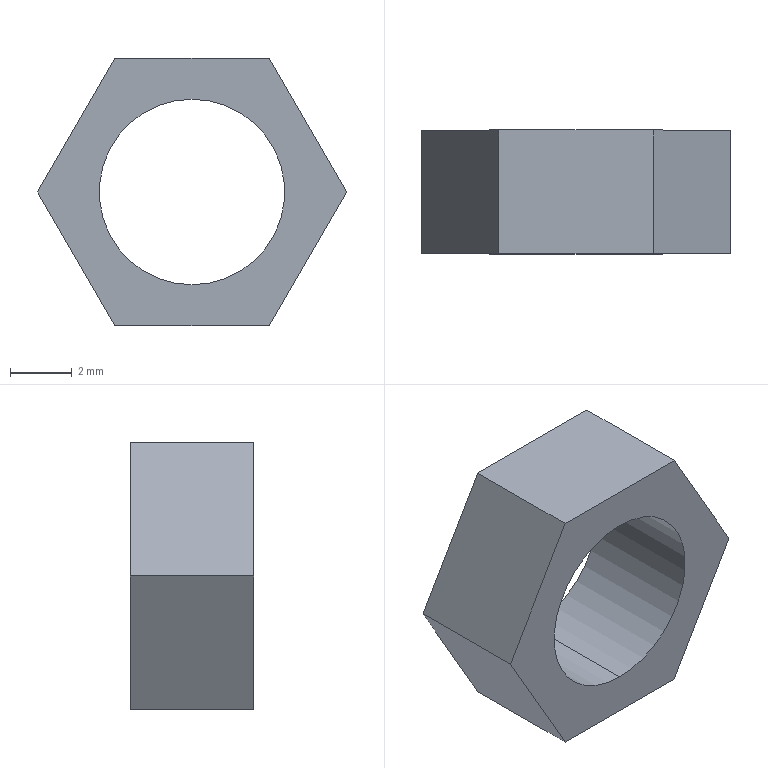Part | NX | features BREP 1 | 1 solid | 10 faces | box 10 x 4 x 8.66 mm | volume 146.71 mm3 | plane 8 | cylinder 2 | commonest cylinder face diameters 6 x2
STEP:
#1=CARTESIAN_POINT('',(0.,0.,-3.));
#2=VERTEX_POINT('',#1);
#3=CARTESIAN_POINT('',(0.,0.,3.));
#4=VERTEX_POINT('',#3);
#5=CARTESIAN_POINT('',(0.,0.,0.));
#6=DIRECTION('',(0.,1.,0.));
#7=DIRECTION('',(0.,0.,1.));
#8=AXIS2_PLACEMENT_3D('',#5,#6,#7);
#9=CIRCLE('',#8,3.);
#10=EDGE_CURVE('',#2,#4,#9,.T.);
#11=ORIENTED_EDGE('',*,*,#10,.F.);
#12=CARTESIAN_POINT('',(0.,4.,-3.));
#13=VERTEX_POINT('',#12);
#14=CARTESIAN_POINT('',(0.,0.,-3.));
#15=DIRECTION('',(0.,1.,0.));
#16=VECTOR('',#15,1000.);
#17=LINE('',#14,#16);
#18=EDGE_CURVE('',#2,#13,#17,.T.);
#19=ORIENTED_EDGE('',*,*,#18,.T.);
#20=CARTESIAN_POINT('',(0.,4.,3.));
#21=VERTEX_POINT('',#20);
#22=CARTESIAN_POINT('',(0.,4.,0.));
#23=DIRECTION('',(0.,1.,0.));
#24=DIRECTION('',(0.,0.,1.));
#25=AXIS2_PLACEMENT_3D('',#22,#23,#24);
#26=CIRCLE('',#25,3.);
#27=EDGE_CURVE('',#13,#21,#26,.T.);
#28=ORIENTED_EDGE('',*,*,#27,.T.);
#29=CARTESIAN_POINT('',(0.,0.,3.));
#30=DIRECTION('',(0.,1.,0.));
#31=VECTOR('',#30,1000.);
#32=LINE('',#29,#31);
#33=EDGE_CURVE('',#4,#21,#32,.T.);
#34=ORIENTED_EDGE('',*,*,#33,.F.);
#35=EDGE_LOOP('',(#11,#19,#28,#34));
#36=FACE_BOUND('',#35,.T.);
#37=CARTESIAN_POINT('',(0.,0.,0.));
#38=DIRECTION('',(0.,1.,0.));
#39=DIRECTION('',(0.,0.,-1.));
#40=AXIS2_PLACEMENT_3D('',#37,#38,#39);
#41=CYLINDRICAL_SURFACE('',#40,3.);
#42=ADVANCED_FACE('',(#36),#41,.F.);
#43=CARTESIAN_POINT('',(2.5,0.,4.33));
#44=VERTEX_POINT('',#43);
#45=CARTESIAN_POINT('',(5.,0.,0.));
#46=VERTEX_POINT('',#45);
#47=CARTESIAN_POINT('',(2.5,0.,4.33));
#48=DIRECTION('',(0.5,0.,-0.866));
#49=VECTOR('',#48,1000.);
#50=LINE('',#47,#49);
#51=EDGE_CURVE('',#44,#46,#50,.T.);
#52=ORIENTED_EDGE('',*,*,#51,.T.);
#53=CARTESIAN_POINT('',(5.,4.,0.));
#54=VERTEX_POINT('',#53);
#55=CARTESIAN_POINT('',(5.,4.,0.));
#56=DIRECTION('',(0.,-1.,0.));
#57=VECTOR('',#56,1000.);
#58=LINE('',#55,#57);
#59=EDGE_CURVE('',#54,#46,#58,.T.);
#60=ORIENTED_EDGE('',*,*,#59,.F.);
#61=CARTESIAN_POINT('',(2.5,4.,4.33));
#62=VERTEX_POINT('',#61);
#63=CARTESIAN_POINT('',(2.5,4.,4.33));
#64=DIRECTION('',(0.5,0.,-0.866));
#65=VECTOR('',#64,1000.);
#66=LINE('',#63,#65);
#67=EDGE_CURVE('',#62,#54,#66,.T.);
#68=ORIENTED_EDGE('',*,*,#67,.F.);
#69=CARTESIAN_POINT('',(2.5,4.,4.33));
#70=DIRECTION('',(0.,-1.,0.));
#71=VECTOR('',#70,1000.);
#72=LINE('',#69,#71);
#73=EDGE_CURVE('',#62,#44,#72,.T.);
#74=ORIENTED_EDGE('',*,*,#73,.T.);
#75=EDGE_LOOP('',(#52,#60,#68,#74));
#76=FACE_BOUND('',#75,.T.);
#77=CARTESIAN_POINT('',(2.5,4.,4.33));
#78=DIRECTION('',(-0.866,0.,-0.5));
#79=DIRECTION('',(0.5,0.,-0.866));
#80=AXIS2_PLACEMENT_3D('',#77,#78,#79);
#81=PLANE('',#80);
#82=ADVANCED_FACE('',(#76),#81,.F.);
#83=CARTESIAN_POINT('',(2.5,0.,-4.33));
#84=VERTEX_POINT('',#83);
#85=CARTESIAN_POINT('',(5.,0.,0.));
#86=DIRECTION('',(-0.5,0.,-0.866));
#87=VECTOR('',#86,1000.);
#88=LINE('',#85,#87);
#89=EDGE_CURVE('',#46,#84,#88,.T.);
#90=ORIENTED_EDGE('',*,*,#89,.T.);
#91=CARTESIAN_POINT('',(2.5,4.,-4.33));
#92=VERTEX_POINT('',#91);
#93=CARTESIAN_POINT('',(2.5,4.,-4.33));
#94=DIRECTION('',(0.,-1.,0.));
#95=VECTOR('',#94,1000.);
#96=LINE('',#93,#95);
#97=EDGE_CURVE('',#92,#84,#96,.T.);
#98=ORIENTED_EDGE('',*,*,#97,.F.);
#99=CARTESIAN_POINT('',(5.,4.,0.));
#100=DIRECTION('',(-0.5,0.,-0.866));
#101=VECTOR('',#100,1000.);
#102=LINE('',#99,#101);
#103=EDGE_CURVE('',#54,#92,#102,.T.);
#104=ORIENTED_EDGE('',*,*,#103,.F.);
#105=ORIENTED_EDGE('',*,*,#59,.T.);
#106=EDGE_LOOP('',(#90,#98,#104,#105));
#107=FACE_BOUND('',#106,.T.);
#108=CARTESIAN_POINT('',(5.,4.,0.));
#109=DIRECTION('',(-0.866,0.,0.5));
#110=DIRECTION('',(0.,-1.,0.));
#111=AXIS2_PLACEMENT_3D('',#108,#109,#110);
#112=PLANE('',#111);
#113=ADVANCED_FACE('',(#107),#112,.F.);
#114=CARTESIAN_POINT('',(-2.5,0.,-4.33));
#115=VERTEX_POINT('',#114);
#116=CARTESIAN_POINT('',(2.5,0.,-4.33));
#117=DIRECTION('',(-1.,0.,0.));
#118=VECTOR('',#117,1000.);
#119=LINE('',#116,#118);
#120=EDGE_CURVE('',#84,#115,#119,.T.);
#121=ORIENTED_EDGE('',*,*,#120,.T.);
#122=CARTESIAN_POINT('',(-2.5,4.,-4.33));
#123=VERTEX_POINT('',#122);
#124=CARTESIAN_POINT('',(-2.5,4.,-4.33));
#125=DIRECTION('',(0.,-1.,0.));
#126=VECTOR('',#125,1000.);
#127=LINE('',#124,#126);
#128=EDGE_CURVE('',#123,#115,#127,.T.);
#129=ORIENTED_EDGE('',*,*,#128,.F.);
#130=CARTESIAN_POINT('',(2.5,4.,-4.33));
#131=DIRECTION('',(-1.,0.,0.));
#132=VECTOR('',#131,1000.);
#133=LINE('',#130,#132);
#134=EDGE_CURVE('',#92,#123,#133,.T.);
#135=ORIENTED_EDGE('',*,*,#134,.F.);
#136=ORIENTED_EDGE('',*,*,#97,.T.);
#137=EDGE_LOOP('',(#121,#129,#135,#136));
#138=FACE_BOUND('',#137,.T.);
#139=CARTESIAN_POINT('',(2.5,4.,-4.33));
#140=DIRECTION('',(0.,0.,1.));
#141=DIRECTION('',(-1.,0.,0.));
#142=AXIS2_PLACEMENT_3D('',#139,#140,#141);
#143=PLANE('',#142);
#144=ADVANCED_FACE('',(#138),#143,.F.);
#145=CARTESIAN_POINT('',(-5.,0.,0.));
#146=VERTEX_POINT('',#145);
#147=CARTESIAN_POINT('',(-2.5,0.,-4.33));
#148=DIRECTION('',(-0.5,0.,0.866));
#149=VECTOR('',#148,1000.);
#150=LINE('',#147,#149);
#151=EDGE_CURVE('',#115,#146,#150,.T.);
#152=ORIENTED_EDGE('',*,*,#151,.T.);
#153=CARTESIAN_POINT('',(-5.,4.,0.));
#154=VERTEX_POINT('',#153);
#155=CARTESIAN_POINT('',(-5.,4.,0.));
#156=DIRECTION('',(0.,-1.,0.));
#157=VECTOR('',#156,1000.);
#158=LINE('',#155,#157);
#159=EDGE_CURVE('',#154,#146,#158,.T.);
#160=ORIENTED_EDGE('',*,*,#159,.F.);
#161=CARTESIAN_POINT('',(-2.5,4.,-4.33));
#162=DIRECTION('',(-0.5,0.,0.866));
#163=VECTOR('',#162,1000.);
#164=LINE('',#161,#163);
#165=EDGE_CURVE('',#123,#154,#164,.T.);
#166=ORIENTED_EDGE('',*,*,#165,.F.);
#167=ORIENTED_EDGE('',*,*,#128,.T.);
#168=EDGE_LOOP('',(#152,#160,#166,#167));
#169=FACE_BOUND('',#168,.T.);
#170=CARTESIAN_POINT('',(-2.5,4.,-4.33));
#171=DIRECTION('',(0.866,0.,0.5));
#172=DIRECTION('',(0.,1.,0.));
#173=AXIS2_PLACEMENT_3D('',#170,#171,#172);
#174=PLANE('',#173);
#175=ADVANCED_FACE('',(#169),#174,.F.);
#176=CARTESIAN_POINT('',(-2.5,0.,4.33));
#177=VERTEX_POINT('',#176);
#178=CARTESIAN_POINT('',(-5.,0.,0.));
#179=DIRECTION('',(0.5,0.,0.866));
#180=VECTOR('',#179,1000.);
#181=LINE('',#178,#180);
#182=EDGE_CURVE('',#146,#177,#181,.T.);
#183=ORIENTED_EDGE('',*,*,#182,.T.);
#184=CARTESIAN_POINT('',(-2.5,4.,4.33));
#185=VERTEX_POINT('',#184);
#186=CARTESIAN_POINT('',(-2.5,4.,4.33));
#187=DIRECTION('',(0.,-1.,0.));
#188=VECTOR('',#187,1000.);
#189=LINE('',#186,#188);
#190=EDGE_CURVE('',#185,#177,#189,.T.);
#191=ORIENTED_EDGE('',*,*,#190,.F.);
#192=CARTESIAN_POINT('',(-5.,4.,0.));
#193=DIRECTION('',(0.5,0.,0.866));
#194=VECTOR('',#193,1000.);
#195=LINE('',#192,#194);
#196=EDGE_CURVE('',#154,#185,#195,.T.);
#197=ORIENTED_EDGE('',*,*,#196,.F.);
#198=ORIENTED_EDGE('',*,*,#159,.T.);
#199=EDGE_LOOP('',(#183,#191,#197,#198));
#200=FACE_BOUND('',#199,.T.);
#201=CARTESIAN_POINT('',(-5.,4.,0.));
#202=DIRECTION('',(0.866,0.,-0.5));
#203=DIRECTION('',(0.,1.,0.));
#204=AXIS2_PLACEMENT_3D('',#201,#202,#203);
#205=PLANE('',#204);
#206=ADVANCED_FACE('',(#200),#205,.F.);
#207=CARTESIAN_POINT('',(-2.5,0.,4.33));
#208=DIRECTION('',(1.,0.,0.));
#209=VECTOR('',#208,1000.);
#210=LINE('',#207,#209);
#211=EDGE_CURVE('',#177,#44,#210,.T.);
#212=ORIENTED_EDGE('',*,*,#211,.T.);
#213=ORIENTED_EDGE('',*,*,#73,.F.);
#214=CARTESIAN_POINT('',(-2.5,4.,4.33));
#215=DIRECTION('',(1.,0.,0.));
#216=VECTOR('',#215,1000.);
#217=LINE('',#214,#216);
#218=EDGE_CURVE('',#185,#62,#217,.T.);
#219=ORIENTED_EDGE('',*,*,#218,.F.);
#220=ORIENTED_EDGE('',*,*,#190,.T.);
#221=EDGE_LOOP('',(#212,#213,#219,#220));
#222=FACE_BOUND('',#221,.T.);
#223=CARTESIAN_POINT('',(-2.5,4.,4.33));
#224=DIRECTION('',(0.,0.,-1.));
#225=DIRECTION('',(1.,0.,0.));
#226=AXIS2_PLACEMENT_3D('',#223,#224,#225);
#227=PLANE('',#226);
#228=ADVANCED_FACE('',(#222),#227,.F.);
#229=ORIENTED_EDGE('',*,*,#67,.T.);
#230=ORIENTED_EDGE('',*,*,#103,.T.);
#231=ORIENTED_EDGE('',*,*,#134,.T.);
#232=ORIENTED_EDGE('',*,*,#165,.T.);
#233=ORIENTED_EDGE('',*,*,#196,.T.);
#234=ORIENTED_EDGE('',*,*,#218,.T.);
#235=EDGE_LOOP('',(#229,#230,#231,#232,#233,#234));
#236=FACE_BOUND('',#235,.T.);
#237=CARTESIAN_POINT('',(0.,4.,0.));
#238=DIRECTION('',(0.,1.,0.));
#239=DIRECTION('',(0.,0.,1.));
#240=AXIS2_PLACEMENT_3D('',#237,#238,#239);
#241=CIRCLE('',#240,3.);
#242=EDGE_CURVE('',#21,#13,#241,.T.);
#243=ORIENTED_EDGE('',*,*,#242,.F.);
#244=ORIENTED_EDGE('',*,*,#27,.F.);
#245=EDGE_LOOP('',(#243,#244));
#246=FACE_BOUND('',#245,.T.);
#247=CARTESIAN_POINT('',(0.,4.,0.));
#248=DIRECTION('',(0.,1.,0.));
#249=DIRECTION('',(0.,0.,1.));
#250=AXIS2_PLACEMENT_3D('',#247,#248,#249);
#251=PLANE('',#250);
#252=ADVANCED_FACE('',(#236,#246),#251,.T.);
#253=ORIENTED_EDGE('',*,*,#51,.F.);
#254=ORIENTED_EDGE('',*,*,#211,.F.);
#255=ORIENTED_EDGE('',*,*,#182,.F.);
#256=ORIENTED_EDGE('',*,*,#151,.F.);
#257=ORIENTED_EDGE('',*,*,#120,.F.);
#258=ORIENTED_EDGE('',*,*,#89,.F.);
#259=EDGE_LOOP('',(#253,#254,#255,#256,#257,#258));
#260=FACE_BOUND('',#259,.T.);
#261=CARTESIAN_POINT('',(0.,0.,0.));
#262=DIRECTION('',(0.,1.,0.));
#263=DIRECTION('',(0.,0.,1.));
#264=AXIS2_PLACEMENT_3D('',#261,#262,#263);
#265=CIRCLE('',#264,3.);
#266=EDGE_CURVE('',#4,#2,#265,.T.);
#267=ORIENTED_EDGE('',*,*,#266,.T.);
#268=ORIENTED_EDGE('',*,*,#10,.T.);
#269=EDGE_LOOP('',(#267,#268));
#270=FACE_BOUND('',#269,.T.);
#271=CARTESIAN_POINT('',(0.,0.,0.));
#272=DIRECTION('',(0.,1.,0.));
#273=DIRECTION('',(0.,0.,1.));
#274=AXIS2_PLACEMENT_3D('',#271,#272,#273);
#275=PLANE('',#274);
#276=ADVANCED_FACE('',(#260,#270),#275,.F.);
#277=ORIENTED_EDGE('',*,*,#18,.F.);
#278=ORIENTED_EDGE('',*,*,#266,.F.);
#279=ORIENTED_EDGE('',*,*,#33,.T.);
#280=ORIENTED_EDGE('',*,*,#242,.T.);
#281=EDGE_LOOP('',(#277,#278,#279,#280));
#282=FACE_BOUND('',#281,.T.);
#283=CARTESIAN_POINT('',(0.,0.,0.));
#284=DIRECTION('',(0.,1.,0.));
#285=DIRECTION('',(0.,0.,-1.));
#286=AXIS2_PLACEMENT_3D('',#283,#284,#285);
#287=CYLINDRICAL_SURFACE('',#286,3.);
#288=ADVANCED_FACE('',(#282),#287,.F.);
#289=CLOSED_SHELL('',(#42,#82,#113,#144,#175,#206,#228,#252,#276,#288));
#290=MANIFOLD_SOLID_BREP('',#289);
#291=(LENGTH_UNIT()NAMED_UNIT(*)SI_UNIT(.MILLI.,.METRE.));
#292=UNCERTAINTY_MEASURE_WITH_UNIT(LENGTH_MEASURE(0.00001),#291,'','');
#293=(NAMED_UNIT(*)PLANE_ANGLE_UNIT()SI_UNIT($,.RADIAN.));
#294=(NAMED_UNIT(*)SI_UNIT($,.STERADIAN.)SOLID_ANGLE_UNIT());
#295=(GEOMETRIC_REPRESENTATION_CONTEXT(3)GLOBAL_UNCERTAINTY_ASSIGNED_CONTEXT((#292))GLOBAL_UNIT_ASSIGNED_CONTEXT((#291,#293,#294))REPRESENTATION_CONTEXT('',''));
#296=ADVANCED_BREP_SHAPE_REPRESENTATION('',(#290),#295);